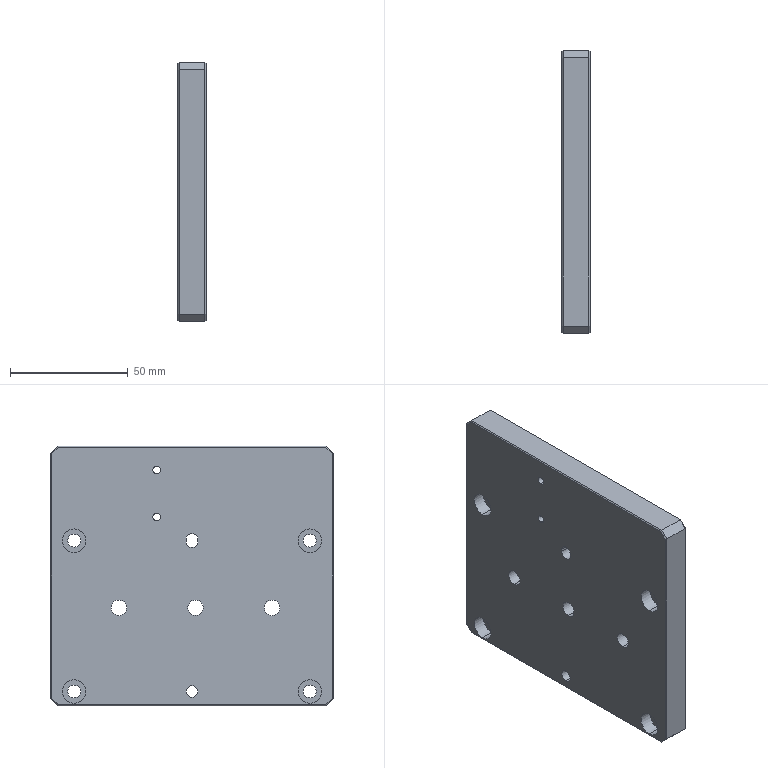Part | STEP file | HJDX-002 | 1 solid | 72 faces | box 12 x 120 x 110 mm | volume 152611 mm3 | cylinder 37 | plane 35 | commonest cylinder face diameters 5.5 x8 10 x8 6.6 x6 11 x6 5 x5 3.3 x4